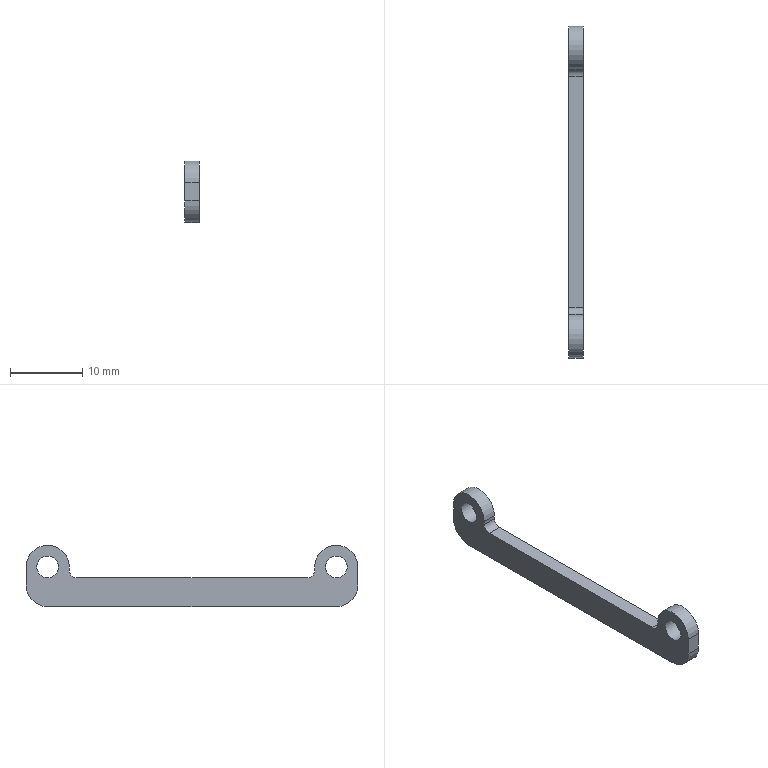Part | STEP file | 1-53.3 | 1 solid | 16 faces | box 2 x 46 x 8.5 mm | volume 425.407 mm3 | cylinder 8 | plane 8 | commonest cylinder face diameters 6 x4 2 x2 3 x2
STEP:
#1=CARTESIAN_POINT('',(0.,0.,0.));
#2=DIRECTION('',(0.,0.,1.));
#3=DIRECTION('',(1.,0.,0.));
#4=AXIS2_PLACEMENT_3D('',#1,#2,#3);
#5=CARTESIAN_POINT('',(-1.,-17.,0.));
#6=VERTEX_POINT('',#5);
#7=CARTESIAN_POINT('',(-1.,-23.,0.));
#8=VERTEX_POINT('',#7);
#9=CARTESIAN_POINT('',(-1.,-20.,0.));
#10=DIRECTION('',(1.,0.,0.));
#11=DIRECTION('',(0.,1.,0.));
#12=AXIS2_PLACEMENT_3D('',#9,#10,#11);
#13=CIRCLE('',#12,3.);
#14=CARTESIAN_POINT('',(-1.,-20.,0.));
#15=DIRECTION('',(1.,0.,0.));
#16=DIRECTION('',(0.,1.,0.));
#17=AXIS2_PLACEMENT_3D('',#14,#15,#16);
#18=CYLINDRICAL_SURFACE('',#17,3.);
#19=CARTESIAN_POINT('',(0.,0.));
#20=DIRECTION('',(1.,0.));
#21=VECTOR('',#20,1.);
#22=LINE('',#19,#21);
#23=(GEOMETRIC_REPRESENTATION_CONTEXT(2)PARAMETRIC_REPRESENTATION_CONTEXT()REPRESENTATION_CONTEXT('',''));
#24=DEFINITIONAL_REPRESENTATION('',(#22),#23);
#25=PCURVE('',#18,#24);
#26=CARTESIAN_POINT('',(-1.,0.,17.5));
#27=DIRECTION('',(1.,0.,0.));
#28=DIRECTION('',(0.,1.,0.));
#29=AXIS2_PLACEMENT_3D('',#26,#27,#28);
#30=PLANE('',#29);
#31=CARTESIAN_POINT('',(-20.,-17.5));
#32=DIRECTION('',(1.,0.));
#33=AXIS2_PLACEMENT_2D('',#31,#32);
#34=CIRCLE('',#33,3.);
#35=(GEOMETRIC_REPRESENTATION_CONTEXT(2)PARAMETRIC_REPRESENTATION_CONTEXT()REPRESENTATION_CONTEXT('',''));
#36=DEFINITIONAL_REPRESENTATION('',(#34),#35);
#37=PCURVE('',#30,#36);
#38=SURFACE_CURVE('',#13,(#25,#37),.PCURVE_S1.);
#39=EDGE_CURVE('',#6,#8,#38,.T.);
#40=ORIENTED_EDGE('',*,*,#39,.T.);
#41=CARTESIAN_POINT('',(1.,-23.,0.));
#42=VERTEX_POINT('',#41);
#43=CARTESIAN_POINT('',(-1.,-23.,0.));
#44=DIRECTION('',(1.,0.,0.));
#45=VECTOR('',#44,1.);
#46=LINE('',#43,#45);
#47=CARTESIAN_POINT('',(3.142,0.));
#48=DIRECTION('',(0.,1.));
#49=VECTOR('',#48,1.);
#50=LINE('',#47,#49);
#51=(GEOMETRIC_REPRESENTATION_CONTEXT(2)PARAMETRIC_REPRESENTATION_CONTEXT()REPRESENTATION_CONTEXT('',''));
#52=DEFINITIONAL_REPRESENTATION('',(#50),#51);
#53=PCURVE('',#18,#52);
#54=CARTESIAN_POINT('',(0.,-23.,-2.75));
#55=DIRECTION('',(0.,-1.,0.));
#56=DIRECTION('',(0.,0.,-1.));
#57=AXIS2_PLACEMENT_3D('',#54,#55,#56);
#58=PLANE('',#57);
#59=CARTESIAN_POINT('',(-2.75,-1.));
#60=DIRECTION('',(0.,1.));
#61=VECTOR('',#60,1.);
#62=LINE('',#59,#61);
#63=(GEOMETRIC_REPRESENTATION_CONTEXT(2)PARAMETRIC_REPRESENTATION_CONTEXT()REPRESENTATION_CONTEXT('',''));
#64=DEFINITIONAL_REPRESENTATION('',(#62),#63);
#65=PCURVE('',#58,#64);
#66=SURFACE_CURVE('',#46,(#53,#65),.PCURVE_S1.);
#67=EDGE_CURVE('',#8,#42,#66,.T.);
#68=ORIENTED_EDGE('',*,*,#67,.T.);
#69=CARTESIAN_POINT('',(1.,-17.,0.));
#70=VERTEX_POINT('',#69);
#71=CARTESIAN_POINT('',(1.,-20.,0.));
#72=DIRECTION('',(1.,0.,0.));
#73=DIRECTION('',(0.,1.,0.));
#74=AXIS2_PLACEMENT_3D('',#71,#72,#73);
#75=CIRCLE('',#74,3.);
#76=CARTESIAN_POINT('',(0.,2.));
#77=DIRECTION('',(1.,0.));
#78=VECTOR('',#77,1.);
#79=LINE('',#76,#78);
#80=(GEOMETRIC_REPRESENTATION_CONTEXT(2)PARAMETRIC_REPRESENTATION_CONTEXT()REPRESENTATION_CONTEXT('',''));
#81=DEFINITIONAL_REPRESENTATION('',(#79),#80);
#82=PCURVE('',#18,#81);
#83=CARTESIAN_POINT('',(1.,0.,17.5));
#84=DIRECTION('',(1.,0.,0.));
#85=DIRECTION('',(0.,1.,0.));
#86=AXIS2_PLACEMENT_3D('',#83,#84,#85);
#87=PLANE('',#86);
#88=CARTESIAN_POINT('',(-20.,-17.5));
#89=DIRECTION('',(1.,0.));
#90=AXIS2_PLACEMENT_2D('',#88,#89);
#91=CIRCLE('',#90,3.);
#92=(GEOMETRIC_REPRESENTATION_CONTEXT(2)PARAMETRIC_REPRESENTATION_CONTEXT()REPRESENTATION_CONTEXT('',''));
#93=DEFINITIONAL_REPRESENTATION('',(#91),#92);
#94=PCURVE('',#87,#93);
#95=SURFACE_CURVE('',#75,(#82,#94),.PCURVE_S1.);
#96=EDGE_CURVE('',#70,#42,#95,.T.);
#97=ORIENTED_EDGE('',*,*,#96,.F.);
#98=CARTESIAN_POINT('',(-1.,-17.,0.));
#99=DIRECTION('',(1.,0.,0.));
#100=VECTOR('',#99,1.);
#101=LINE('',#98,#100);
#102=CARTESIAN_POINT('',(0.,0.));
#103=DIRECTION('',(0.,1.));
#104=VECTOR('',#103,1.);
#105=LINE('',#102,#104);
#106=(GEOMETRIC_REPRESENTATION_CONTEXT(2)PARAMETRIC_REPRESENTATION_CONTEXT()REPRESENTATION_CONTEXT('',''));
#107=DEFINITIONAL_REPRESENTATION('',(#105),#106);
#108=PCURVE('',#18,#107);
#109=CARTESIAN_POINT('',(0.,-17.,-0.75));
#110=DIRECTION('',(0.,1.,0.));
#111=DIRECTION('',(0.,0.,1.));
#112=AXIS2_PLACEMENT_3D('',#109,#110,#111);
#113=PLANE('',#112);
#114=CARTESIAN_POINT('',(0.75,-1.));
#115=DIRECTION('',(0.,1.));
#116=VECTOR('',#115,1.);
#117=LINE('',#114,#116);
#118=(GEOMETRIC_REPRESENTATION_CONTEXT(2)PARAMETRIC_REPRESENTATION_CONTEXT()REPRESENTATION_CONTEXT('',''));
#119=DEFINITIONAL_REPRESENTATION('',(#117),#118);
#120=PCURVE('',#113,#119);
#121=SURFACE_CURVE('',#101,(#108,#120),.PCURVE_S1.);
#122=EDGE_CURVE('',#6,#70,#121,.T.);
#123=ORIENTED_EDGE('',*,*,#122,.F.);
#124=EDGE_LOOP('',(#40,#68,#97,#123));
#125=FACE_BOUND('',#124,.T.);
#126=ADVANCED_FACE('',(#125),#18,.T.);
#127=CARTESIAN_POINT('',(-1.,23.,0.));
#128=VERTEX_POINT('',#127);
#129=CARTESIAN_POINT('',(-1.,17.,0.));
#130=VERTEX_POINT('',#129);
#131=CARTESIAN_POINT('',(-1.,20.,0.));
#132=DIRECTION('',(1.,0.,0.));
#133=DIRECTION('',(0.,1.,0.));
#134=AXIS2_PLACEMENT_3D('',#131,#132,#133);
#135=CIRCLE('',#134,3.);
#136=CARTESIAN_POINT('',(-1.,20.,0.));
#137=DIRECTION('',(1.,0.,0.));
#138=DIRECTION('',(0.,1.,0.));
#139=AXIS2_PLACEMENT_3D('',#136,#137,#138);
#140=CYLINDRICAL_SURFACE('',#139,3.);
#141=CARTESIAN_POINT('',(0.,0.));
#142=DIRECTION('',(1.,0.));
#143=VECTOR('',#142,1.);
#144=LINE('',#141,#143);
#145=(GEOMETRIC_REPRESENTATION_CONTEXT(2)PARAMETRIC_REPRESENTATION_CONTEXT()REPRESENTATION_CONTEXT('',''));
#146=DEFINITIONAL_REPRESENTATION('',(#144),#145);
#147=PCURVE('',#140,#146);
#148=CARTESIAN_POINT('',(20.,-17.5));
#149=DIRECTION('',(1.,0.));
#150=AXIS2_PLACEMENT_2D('',#148,#149);
#151=CIRCLE('',#150,3.);
#152=(GEOMETRIC_REPRESENTATION_CONTEXT(2)PARAMETRIC_REPRESENTATION_CONTEXT()REPRESENTATION_CONTEXT('',''));
#153=DEFINITIONAL_REPRESENTATION('',(#151),#152);
#154=PCURVE('',#30,#153);
#155=SURFACE_CURVE('',#135,(#147,#154),.PCURVE_S1.);
#156=EDGE_CURVE('',#128,#130,#155,.T.);
#157=ORIENTED_EDGE('',*,*,#156,.T.);
#158=CARTESIAN_POINT('',(1.,17.,0.));
#159=VERTEX_POINT('',#158);
#160=CARTESIAN_POINT('',(-1.,17.,0.));
#161=DIRECTION('',(1.,0.,0.));
#162=VECTOR('',#161,1.);
#163=LINE('',#160,#162);
#164=CARTESIAN_POINT('',(3.142,0.));
#165=DIRECTION('',(0.,1.));
#166=VECTOR('',#165,1.);
#167=LINE('',#164,#166);
#168=(GEOMETRIC_REPRESENTATION_CONTEXT(2)PARAMETRIC_REPRESENTATION_CONTEXT()REPRESENTATION_CONTEXT('',''));
#169=DEFINITIONAL_REPRESENTATION('',(#167),#168);
#170=PCURVE('',#140,#169);
#171=CARTESIAN_POINT('',(0.,17.,-0.75));
#172=DIRECTION('',(0.,-1.,0.));
#173=DIRECTION('',(0.,0.,-1.));
#174=AXIS2_PLACEMENT_3D('',#171,#172,#173);
#175=PLANE('',#174);
#176=CARTESIAN_POINT('',(-0.75,-1.));
#177=DIRECTION('',(0.,1.));
#178=VECTOR('',#177,1.);
#179=LINE('',#176,#178);
#180=(GEOMETRIC_REPRESENTATION_CONTEXT(2)PARAMETRIC_REPRESENTATION_CONTEXT()REPRESENTATION_CONTEXT('',''));
#181=DEFINITIONAL_REPRESENTATION('',(#179),#180);
#182=PCURVE('',#175,#181);
#183=SURFACE_CURVE('',#163,(#170,#182),.PCURVE_S1.);
#184=EDGE_CURVE('',#130,#159,#183,.T.);
#185=ORIENTED_EDGE('',*,*,#184,.T.);
#186=CARTESIAN_POINT('',(1.,23.,0.));
#187=VERTEX_POINT('',#186);
#188=CARTESIAN_POINT('',(1.,20.,0.));
#189=DIRECTION('',(1.,0.,0.));
#190=DIRECTION('',(0.,1.,0.));
#191=AXIS2_PLACEMENT_3D('',#188,#189,#190);
#192=CIRCLE('',#191,3.);
#193=CARTESIAN_POINT('',(0.,2.));
#194=DIRECTION('',(1.,0.));
#195=VECTOR('',#194,1.);
#196=LINE('',#193,#195);
#197=(GEOMETRIC_REPRESENTATION_CONTEXT(2)PARAMETRIC_REPRESENTATION_CONTEXT()REPRESENTATION_CONTEXT('',''));
#198=DEFINITIONAL_REPRESENTATION('',(#196),#197);
#199=PCURVE('',#140,#198);
#200=CARTESIAN_POINT('',(20.,-17.5));
#201=DIRECTION('',(1.,0.));
#202=AXIS2_PLACEMENT_2D('',#200,#201);
#203=CIRCLE('',#202,3.);
#204=(GEOMETRIC_REPRESENTATION_CONTEXT(2)PARAMETRIC_REPRESENTATION_CONTEXT()REPRESENTATION_CONTEXT('',''));
#205=DEFINITIONAL_REPRESENTATION('',(#203),#204);
#206=PCURVE('',#87,#205);
#207=SURFACE_CURVE('',#192,(#199,#206),.PCURVE_S1.);
#208=EDGE_CURVE('',#187,#159,#207,.T.);
#209=ORIENTED_EDGE('',*,*,#208,.F.);
#210=CARTESIAN_POINT('',(-1.,23.,0.));
#211=DIRECTION('',(1.,0.,0.));
#212=VECTOR('',#211,1.);
#213=LINE('',#210,#212);
#214=CARTESIAN_POINT('',(0.,0.));
#215=DIRECTION('',(0.,1.));
#216=VECTOR('',#215,1.);
#217=LINE('',#214,#216);
#218=(GEOMETRIC_REPRESENTATION_CONTEXT(2)PARAMETRIC_REPRESENTATION_CONTEXT()REPRESENTATION_CONTEXT('',''));
#219=DEFINITIONAL_REPRESENTATION('',(#217),#218);
#220=PCURVE('',#140,#219);
#221=CARTESIAN_POINT('',(0.,23.,-2.75));
#222=DIRECTION('',(0.,1.,0.));
#223=DIRECTION('',(0.,0.,1.));
#224=AXIS2_PLACEMENT_3D('',#221,#222,#223);
#225=PLANE('',#224);
#226=CARTESIAN_POINT('',(2.75,-1.));
#227=DIRECTION('',(0.,1.));
#228=VECTOR('',#227,1.);
#229=LINE('',#226,#228);
#230=(GEOMETRIC_REPRESENTATION_CONTEXT(2)PARAMETRIC_REPRESENTATION_CONTEXT()REPRESENTATION_CONTEXT('',''));
#231=DEFINITIONAL_REPRESENTATION('',(#229),#230);
#232=PCURVE('',#225,#231);
#233=SURFACE_CURVE('',#213,(#220,#232),.PCURVE_S1.);
#234=EDGE_CURVE('',#128,#187,#233,.T.);
#235=ORIENTED_EDGE('',*,*,#234,.F.);
#236=EDGE_LOOP('',(#157,#185,#209,#235));
#237=FACE_BOUND('',#236,.T.);
#238=ADVANCED_FACE('',(#237),#140,.T.);
#239=CARTESIAN_POINT('',(-1.,-18.5,0.));
#240=VERTEX_POINT('',#239);
#241=CARTESIAN_POINT('',(1.,-18.5,0.));
#242=VERTEX_POINT('',#241);
#243=CARTESIAN_POINT('',(-1.,-18.5,0.));
#244=DIRECTION('',(1.,0.,0.));
#245=VECTOR('',#244,1.);
#246=LINE('',#243,#245);
#247=CARTESIAN_POINT('',(-1.,-20.,0.));
#248=DIRECTION('',(1.,0.,0.));
#249=DIRECTION('',(0.,1.,0.));
#250=AXIS2_PLACEMENT_3D('',#247,#248,#249);
#251=CYLINDRICAL_SURFACE('',#250,1.5);
#252=CARTESIAN_POINT('',(6.283,0.));
#253=DIRECTION('',(0.,1.));
#254=VECTOR('',#253,1.);
#255=LINE('',#252,#254);
#256=(GEOMETRIC_REPRESENTATION_CONTEXT(2)PARAMETRIC_REPRESENTATION_CONTEXT()REPRESENTATION_CONTEXT('',''));
#257=DEFINITIONAL_REPRESENTATION('',(#255),#256);
#258=PCURVE('',#251,#257);
#259=CARTESIAN_POINT('',(0.,0.));
#260=DIRECTION('',(0.,1.));
#261=VECTOR('',#260,1.);
#262=LINE('',#259,#261);
#263=(GEOMETRIC_REPRESENTATION_CONTEXT(2)PARAMETRIC_REPRESENTATION_CONTEXT()REPRESENTATION_CONTEXT('',''));
#264=DEFINITIONAL_REPRESENTATION('',(#262),#263);
#265=PCURVE('',#251,#264);
#266=SEAM_CURVE('',#246,(#258,#265),.PCURVE_S1.);
#267=EDGE_CURVE('',#240,#242,#266,.T.);
#268=ORIENTED_EDGE('',*,*,#267,.T.);
#269=CARTESIAN_POINT('',(1.,-20.,0.));
#270=DIRECTION('',(-1.,0.,0.));
#271=DIRECTION('',(0.,1.,0.));
#272=AXIS2_PLACEMENT_3D('',#269,#270,#271);
#273=CIRCLE('',#272,1.5);
#274=CARTESIAN_POINT('',(6.283,2.));
#275=DIRECTION('',(-1.,0.));
#276=VECTOR('',#275,1.);
#277=LINE('',#274,#276);
#278=(GEOMETRIC_REPRESENTATION_CONTEXT(2)PARAMETRIC_REPRESENTATION_CONTEXT()REPRESENTATION_CONTEXT('',''));
#279=DEFINITIONAL_REPRESENTATION('',(#277),#278);
#280=PCURVE('',#251,#279);
#281=CARTESIAN_POINT('',(-18.5,-17.5));
#282=CARTESIAN_POINT('',(-18.5,-20.098));
#283=CARTESIAN_POINT('',(-20.75,-18.799));
#284=CARTESIAN_POINT('',(-23.,-17.5));
#285=CARTESIAN_POINT('',(-20.75,-16.201));
#286=CARTESIAN_POINT('',(-18.5,-14.902));
#287=CARTESIAN_POINT('',(-18.5,-17.5));
#288=(BOUNDED_CURVE()B_SPLINE_CURVE(2,(#281,#282,#283,#284,#285,#286,#287),.UNSPECIFIED.,.T.,.F.)B_SPLINE_CURVE_WITH_KNOTS((1,2,2,2,2,1),(-2.094,0.,2.094,4.189,6.283,8.378),.UNSPECIFIED.)CURVE()GEOMETRIC_REPRESENTATION_ITEM()RATIONAL_B_SPLINE_CURVE((1.,0.5,1.,0.5,1.,0.5,1.))REPRESENTATION_ITEM(''));
#289=(GEOMETRIC_REPRESENTATION_CONTEXT(2)PARAMETRIC_REPRESENTATION_CONTEXT()REPRESENTATION_CONTEXT('',''));
#290=DEFINITIONAL_REPRESENTATION('',(#288),#289);
#291=PCURVE('',#87,#290);
#292=SURFACE_CURVE('',#273,(#280,#291),.PCURVE_S1.);
#293=EDGE_CURVE('',#242,#242,#292,.T.);
#294=ORIENTED_EDGE('',*,*,#293,.T.);
#295=ORIENTED_EDGE('',*,*,#267,.F.);
#296=CARTESIAN_POINT('',(-1.,-20.,0.));
#297=DIRECTION('',(-1.,0.,0.));
#298=DIRECTION('',(0.,1.,0.));
#299=AXIS2_PLACEMENT_3D('',#296,#297,#298);
#300=CIRCLE('',#299,1.5);
#301=CARTESIAN_POINT('',(6.283,0.));
#302=DIRECTION('',(-1.,0.));
#303=VECTOR('',#302,1.);
#304=LINE('',#301,#303);
#305=(GEOMETRIC_REPRESENTATION_CONTEXT(2)PARAMETRIC_REPRESENTATION_CONTEXT()REPRESENTATION_CONTEXT('',''));
#306=DEFINITIONAL_REPRESENTATION('',(#304),#305);
#307=PCURVE('',#251,#306);
#308=CARTESIAN_POINT('',(-18.5,-17.5));
#309=CARTESIAN_POINT('',(-18.5,-20.098));
#310=CARTESIAN_POINT('',(-20.75,-18.799));
#311=CARTESIAN_POINT('',(-23.,-17.5));
#312=CARTESIAN_POINT('',(-20.75,-16.201));
#313=CARTESIAN_POINT('',(-18.5,-14.902));
#314=CARTESIAN_POINT('',(-18.5,-17.5));
#315=(BOUNDED_CURVE()B_SPLINE_CURVE(2,(#308,#309,#310,#311,#312,#313,#314),.UNSPECIFIED.,.T.,.F.)B_SPLINE_CURVE_WITH_KNOTS((1,2,2,2,2,1),(-2.094,0.,2.094,4.189,6.283,8.378),.UNSPECIFIED.)CURVE()GEOMETRIC_REPRESENTATION_ITEM()RATIONAL_B_SPLINE_CURVE((1.,0.5,1.,0.5,1.,0.5,1.))REPRESENTATION_ITEM(''));
#316=(GEOMETRIC_REPRESENTATION_CONTEXT(2)PARAMETRIC_REPRESENTATION_CONTEXT()REPRESENTATION_CONTEXT('',''));
#317=DEFINITIONAL_REPRESENTATION('',(#315),#316);
#318=PCURVE('',#30,#317);
#319=SURFACE_CURVE('',#300,(#307,#318),.PCURVE_S1.);
#320=EDGE_CURVE('',#240,#240,#319,.T.);
#321=ORIENTED_EDGE('',*,*,#320,.F.);
#322=EDGE_LOOP('',(#268,#294,#295,#321));
#323=FACE_BOUND('',#322,.F.);
#324=ADVANCED_FACE('',(#323),#251,.F.);
#325=CARTESIAN_POINT('',(-1.,21.5,0.));
#326=VERTEX_POINT('',#325);
#327=CARTESIAN_POINT('',(1.,21.5,0.));
#328=VERTEX_POINT('',#327);
#329=CARTESIAN_POINT('',(-1.,21.5,0.));
#330=DIRECTION('',(1.,0.,0.));
#331=VECTOR('',#330,1.);
#332=LINE('',#329,#331);
#333=CARTESIAN_POINT('',(-1.,20.,0.));
#334=DIRECTION('',(1.,0.,0.));
#335=DIRECTION('',(0.,1.,0.));
#336=AXIS2_PLACEMENT_3D('',#333,#334,#335);
#337=CYLINDRICAL_SURFACE('',#336,1.5);
#338=CARTESIAN_POINT('',(6.283,0.));
#339=DIRECTION('',(0.,1.));
#340=VECTOR('',#339,1.);
#341=LINE('',#338,#340);
#342=(GEOMETRIC_REPRESENTATION_CONTEXT(2)PARAMETRIC_REPRESENTATION_CONTEXT()REPRESENTATION_CONTEXT('',''));
#343=DEFINITIONAL_REPRESENTATION('',(#341),#342);
#344=PCURVE('',#337,#343);
#345=CARTESIAN_POINT('',(0.,0.));
#346=DIRECTION('',(0.,1.));
#347=VECTOR('',#346,1.);
#348=LINE('',#345,#347);
#349=(GEOMETRIC_REPRESENTATION_CONTEXT(2)PARAMETRIC_REPRESENTATION_CONTEXT()REPRESENTATION_CONTEXT('',''));
#350=DEFINITIONAL_REPRESENTATION('',(#348),#349);
#351=PCURVE('',#337,#350);
#352=SEAM_CURVE('',#332,(#344,#351),.PCURVE_S1.);
#353=EDGE_CURVE('',#326,#328,#352,.T.);
#354=ORIENTED_EDGE('',*,*,#353,.T.);
#355=CARTESIAN_POINT('',(1.,20.,0.));
#356=DIRECTION('',(-1.,0.,0.));
#357=DIRECTION('',(0.,1.,0.));
#358=AXIS2_PLACEMENT_3D('',#355,#356,#357);
#359=CIRCLE('',#358,1.5);
#360=CARTESIAN_POINT('',(6.283,2.));
#361=DIRECTION('',(-1.,0.));
#362=VECTOR('',#361,1.);
#363=LINE('',#360,#362);
#364=(GEOMETRIC_REPRESENTATION_CONTEXT(2)PARAMETRIC_REPRESENTATION_CONTEXT()REPRESENTATION_CONTEXT('',''));
#365=DEFINITIONAL_REPRESENTATION('',(#363),#364);
#366=PCURVE('',#337,#365);
#367=CARTESIAN_POINT('',(21.5,-17.5));
#368=CARTESIAN_POINT('',(21.5,-20.098));
#369=CARTESIAN_POINT('',(19.25,-18.799));
#370=CARTESIAN_POINT('',(17.,-17.5));
#371=CARTESIAN_POINT('',(19.25,-16.201));
#372=CARTESIAN_POINT('',(21.5,-14.902));
#373=CARTESIAN_POINT('',(21.5,-17.5));
#374=(BOUNDED_CURVE()B_SPLINE_CURVE(2,(#367,#368,#369,#370,#371,#372,#373),.UNSPECIFIED.,.T.,.F.)B_SPLINE_CURVE_WITH_KNOTS((1,2,2,2,2,1),(-2.094,0.,2.094,4.189,6.283,8.378),.UNSPECIFIED.)CURVE()GEOMETRIC_REPRESENTATION_ITEM()RATIONAL_B_SPLINE_CURVE((1.,0.5,1.,0.5,1.,0.5,1.))REPRESENTATION_ITEM(''));
#375=(GEOMETRIC_REPRESENTATION_CONTEXT(2)PARAMETRIC_REPRESENTATION_CONTEXT()REPRESENTATION_CONTEXT('',''));
#376=DEFINITIONAL_REPRESENTATION('',(#374),#375);
#377=PCURVE('',#87,#376);
#378=SURFACE_CURVE('',#359,(#366,#377),.PCURVE_S1.);
#379=EDGE_CURVE('',#328,#328,#378,.T.);
#380=ORIENTED_EDGE('',*,*,#379,.T.);
#381=ORIENTED_EDGE('',*,*,#353,.F.);
#382=CARTESIAN_POINT('',(-1.,20.,0.));
#383=DIRECTION('',(-1.,0.,0.));
#384=DIRECTION('',(0.,1.,0.));
#385=AXIS2_PLACEMENT_3D('',#382,#383,#384);
#386=CIRCLE('',#385,1.5);
#387=CARTESIAN_POINT('',(6.283,0.));
#388=DIRECTION('',(-1.,0.));
#389=VECTOR('',#388,1.);
#390=LINE('',#387,#389);
#391=(GEOMETRIC_REPRESENTATION_CONTEXT(2)PARAMETRIC_REPRESENTATION_CONTEXT()REPRESENTATION_CONTEXT('',''));
#392=DEFINITIONAL_REPRESENTATION('',(#390),#391);
#393=PCURVE('',#337,#392);
#394=CARTESIAN_POINT('',(21.5,-17.5));
#395=CARTESIAN_POINT('',(21.5,-20.098));
#396=CARTESIAN_POINT('',(19.25,-18.799));
#397=CARTESIAN_POINT('',(17.,-17.5));
#398=CARTESIAN_POINT('',(19.25,-16.201));
#399=CARTESIAN_POINT('',(21.5,-14.902));
#400=CARTESIAN_POINT('',(21.5,-17.5));
#401=(BOUNDED_CURVE()B_SPLINE_CURVE(2,(#394,#395,#396,#397,#398,#399,#400),.UNSPECIFIED.,.T.,.F.)B_SPLINE_CURVE_WITH_KNOTS((1,2,2,2,2,1),(-2.094,0.,2.094,4.189,6.283,8.378),.UNSPECIFIED.)CURVE()GEOMETRIC_REPRESENTATION_ITEM()RATIONAL_B_SPLINE_CURVE((1.,0.5,1.,0.5,1.,0.5,1.))REPRESENTATION_ITEM(''));
#402=(GEOMETRIC_REPRESENTATION_CONTEXT(2)PARAMETRIC_REPRESENTATION_CONTEXT()REPRESENTATION_CONTEXT('',''));
#403=DEFINITIONAL_REPRESENTATION('',(#401),#402);
#404=PCURVE('',#30,#403);
#405=SURFACE_CURVE('',#386,(#393,#404),.PCURVE_S1.);
#406=EDGE_CURVE('',#326,#326,#405,.T.);
#407=ORIENTED_EDGE('',*,*,#406,.F.);
#408=EDGE_LOOP('',(#354,#380,#381,#407));
#409=FACE_BOUND('',#408,.F.);
#410=ADVANCED_FACE('',(#409),#337,.F.);
#411=CARTESIAN_POINT('',(-1.,-23.,-2.5));
#412=VERTEX_POINT('',#411);
#413=CARTESIAN_POINT('',(-1.,-23.,0.));
#414=DIRECTION('',(0.,0.,-1.));
#415=VECTOR('',#414,1.);
#416=LINE('',#413,#415);
#417=CARTESIAN_POINT('',(-2.75,-1.));
#418=DIRECTION('',(1.,0.));
#419=VECTOR('',#418,1.);
#420=LINE('',#417,#419);
#421=(GEOMETRIC_REPRESENTATION_CONTEXT(2)PARAMETRIC_REPRESENTATION_CONTEXT()REPRESENTATION_CONTEXT('',''));
#422=DEFINITIONAL_REPRESENTATION('',(#420),#421);
#423=PCURVE('',#58,#422);
#424=CARTESIAN_POINT('',(-23.,-17.5));
#425=DIRECTION('',(0.,-1.));
#426=VECTOR('',#425,1.);
#427=LINE('',#424,#426);
#428=(GEOMETRIC_REPRESENTATION_CONTEXT(2)PARAMETRIC_REPRESENTATION_CONTEXT()REPRESENTATION_CONTEXT('',''));
#429=DEFINITIONAL_REPRESENTATION('',(#427),#428);
#430=PCURVE('',#30,#429);
#431=SURFACE_CURVE('',#416,(#423,#430),.PCURVE_S1.);
#432=EDGE_CURVE('',#8,#412,#431,.T.);
#433=ORIENTED_EDGE('',*,*,#432,.T.);
#434=CARTESIAN_POINT('',(1.,-23.,-2.5));
#435=VERTEX_POINT('',#434);
#436=CARTESIAN_POINT('',(-1.,-23.,-2.5));
#437=DIRECTION('',(1.,0.,0.));
#438=VECTOR('',#437,1.);
#439=LINE('',#436,#438);
#440=CARTESIAN_POINT('',(-0.25,-1.));
#441=DIRECTION('',(0.,1.));
#442=VECTOR('',#441,1.);
#443=LINE('',#440,#442);
#444=(GEOMETRIC_REPRESENTATION_CONTEXT(2)PARAMETRIC_REPRESENTATION_CONTEXT()REPRESENTATION_CONTEXT('',''));
#445=DEFINITIONAL_REPRESENTATION('',(#443),#444);
#446=PCURVE('',#58,#445);
#447=CARTESIAN_POINT('',(-1.,-20.,-2.5));
#448=DIRECTION('',(1.,0.,0.));
#449=DIRECTION('',(0.,-1.,0.));
#450=AXIS2_PLACEMENT_3D('',#447,#448,#449);
#451=CYLINDRICAL_SURFACE('',#450,3.);
#452=CARTESIAN_POINT('',(0.,0.));
#453=DIRECTION('',(0.,1.));
#454=VECTOR('',#453,1.);
#455=LINE('',#452,#454);
#456=(GEOMETRIC_REPRESENTATION_CONTEXT(2)PARAMETRIC_REPRESENTATION_CONTEXT()REPRESENTATION_CONTEXT('',''));
#457=DEFINITIONAL_REPRESENTATION('',(#455),#456);
#458=PCURVE('',#451,#457);
#459=SURFACE_CURVE('',#439,(#446,#458),.PCURVE_S1.);
#460=EDGE_CURVE('',#412,#435,#459,.T.);
#461=ORIENTED_EDGE('',*,*,#460,.T.);
#462=CARTESIAN_POINT('',(1.,-23.,0.));
#463=DIRECTION('',(0.,0.,-1.));
#464=VECTOR('',#463,1.);
#465=LINE('',#462,#464);
#466=CARTESIAN_POINT('',(-2.75,1.));
#467=DIRECTION('',(1.,0.));
#468=VECTOR('',#467,1.);
#469=LINE('',#466,#468);
#470=(GEOMETRIC_REPRESENTATION_CONTEXT(2)PARAMETRIC_REPRESENTATION_CONTEXT()REPRESENTATION_CONTEXT('',''));
#471=DEFINITIONAL_REPRESENTATION('',(#469),#470);
#472=PCURVE('',#58,#471);
#473=CARTESIAN_POINT('',(-23.,-17.5));
#474=DIRECTION('',(0.,-1.));
#475=VECTOR('',#474,1.);
#476=LINE('',#473,#475);
#477=(GEOMETRIC_REPRESENTATION_CONTEXT(2)PARAMETRIC_REPRESENTATION_CONTEXT()REPRESENTATION_CONTEXT('',''));
#478=DEFINITIONAL_REPRESENTATION('',(#476),#477);
#479=PCURVE('',#87,#478);
#480=SURFACE_CURVE('',#465,(#472,#479),.PCURVE_S1.);
#481=EDGE_CURVE('',#42,#435,#480,.T.);
#482=ORIENTED_EDGE('',*,*,#481,.F.);
#483=ORIENTED_EDGE('',*,*,#67,.F.);
#484=EDGE_LOOP('',(#433,#461,#482,#483));
#485=FACE_BOUND('',#484,.T.);
#486=ADVANCED_FACE('',(#485),#58,.T.);
#487=CARTESIAN_POINT('',(-1.,-20.,-5.5));
#488=VERTEX_POINT('',#487);
#489=CARTESIAN_POINT('',(-1.,20.,-5.5));
#490=VERTEX_POINT('',#489);
#491=CARTESIAN_POINT('',(-1.,-20.,-5.5));
#492=DIRECTION('',(0.,1.,0.));
#493=VECTOR('',#492,1.);
#494=LINE('',#491,#493);
#495=CARTESIAN_POINT('',(0.,0.,-5.5));
#496=DIRECTION('',(0.,0.,-1.));
#497=DIRECTION('',(0.,1.,0.));
#498=AXIS2_PLACEMENT_3D('',#495,#496,#497);
#499=PLANE('',#498);
#500=CARTESIAN_POINT('',(-20.,-1.));
#501=DIRECTION('',(1.,0.));
#502=VECTOR('',#501,1.);
#503=LINE('',#500,#502);
#504=(GEOMETRIC_REPRESENTATION_CONTEXT(2)PARAMETRIC_REPRESENTATION_CONTEXT()REPRESENTATION_CONTEXT('',''));
#505=DEFINITIONAL_REPRESENTATION('',(#503),#504);
#506=PCURVE('',#499,#505);
#507=CARTESIAN_POINT('',(-20.,-23.));
#508=DIRECTION('',(1.,0.));
#509=VECTOR('',#508,1.);
#510=LINE('',#507,#509);
#511=(GEOMETRIC_REPRESENTATION_CONTEXT(2)PARAMETRIC_REPRESENTATION_CONTEXT()REPRESENTATION_CONTEXT('',''));
#512=DEFINITIONAL_REPRESENTATION('',(#510),#511);
#513=PCURVE('',#30,#512);
#514=SURFACE_CURVE('',#494,(#506,#513),.PCURVE_S1.);
#515=EDGE_CURVE('',#488,#490,#514,.T.);
#516=ORIENTED_EDGE('',*,*,#515,.T.);
#517=CARTESIAN_POINT('',(1.,20.,-5.5));
#518=VERTEX_POINT('',#517);
#519=CARTESIAN_POINT('',(-1.,20.,-5.5));
#520=DIRECTION('',(1.,0.,0.));
#521=VECTOR('',#520,1.);
#522=LINE('',#519,#521);
#523=CARTESIAN_POINT('',(20.,-1.));
#524=DIRECTION('',(0.,1.));
#525=VECTOR('',#524,1.);
#526=LINE('',#523,#525);
#527=(GEOMETRIC_REPRESENTATION_CONTEXT(2)PARAMETRIC_REPRESENTATION_CONTEXT()REPRESENTATION_CONTEXT('',''));
#528=DEFINITIONAL_REPRESENTATION('',(#526),#527);
#529=PCURVE('',#499,#528);
#530=CARTESIAN_POINT('',(-1.,20.,-2.5));
#531=DIRECTION('',(1.,0.,0.));
#532=DIRECTION('',(0.,0.,-1.));
#533=AXIS2_PLACEMENT_3D('',#530,#531,#532);
#534=CYLINDRICAL_SURFACE('',#533,3.);
#535=CARTESIAN_POINT('',(0.,0.));
#536=DIRECTION('',(0.,1.));
#537=VECTOR('',#536,1.);
#538=LINE('',#535,#537);
#539=(GEOMETRIC_REPRESENTATION_CONTEXT(2)PARAMETRIC_REPRESENTATION_CONTEXT()REPRESENTATION_CONTEXT('',''));
#540=DEFINITIONAL_REPRESENTATION('',(#538),#539);
#541=PCURVE('',#534,#540);
#542=SURFACE_CURVE('',#522,(#529,#541),.PCURVE_S1.);
#543=EDGE_CURVE('',#490,#518,#542,.T.);
#544=ORIENTED_EDGE('',*,*,#543,.T.);
#545=CARTESIAN_POINT('',(1.,-20.,-5.5));
#546=VERTEX_POINT('',#545);
#547=CARTESIAN_POINT('',(1.,-20.,-5.5));
#548=DIRECTION('',(0.,1.,0.));
#549=VECTOR('',#548,1.);
#550=LINE('',#547,#549);
#551=CARTESIAN_POINT('',(-20.,1.));
#552=DIRECTION('',(1.,0.));
#553=VECTOR('',#552,1.);
#554=LINE('',#551,#553);
#555=(GEOMETRIC_REPRESENTATION_CONTEXT(2)PARAMETRIC_REPRESENTATION_CONTEXT()REPRESENTATION_CONTEXT('',''));
#556=DEFINITIONAL_REPRESENTATION('',(#554),#555);
#557=PCURVE('',#499,#556);
#558=CARTESIAN_POINT('',(-20.,-23.));
#559=DIRECTION('',(1.,0.));
#560=VECTOR('',#559,1.);
#561=LINE('',#558,#560);
#562=(GEOMETRIC_REPRESENTATION_CONTEXT(2)PARAMETRIC_REPRESENTATION_CONTEXT()REPRESENTATION_CONTEXT('',''));
#563=DEFINITIONAL_REPRESENTATION('',(#561),#562);
#564=PCURVE('',#87,#563);
#565=SURFACE_CURVE('',#550,(#557,#564),.PCURVE_S1.);
#566=EDGE_CURVE('',#546,#518,#565,.T.);
#567=ORIENTED_EDGE('',*,*,#566,.F.);
#568=CARTESIAN_POINT('',(-1.,-20.,-5.5));
#569=DIRECTION('',(1.,0.,0.));
#570=VECTOR('',#569,1.);
#571=LINE('',#568,#570);
#572=CARTESIAN_POINT('',(-20.,-1.));
#573=DIRECTION('',(0.,1.));
#574=VECTOR('',#573,1.);
#575=LINE('',#572,#574);
#576=(GEOMETRIC_REPRESENTATION_CONTEXT(2)PARAMETRIC_REPRESENTATION_CONTEXT()REPRESENTATION_CONTEXT('',''));
#577=DEFINITIONAL_REPRESENTATION('',(#575),#576);
#578=PCURVE('',#499,#577);
#579=CARTESIAN_POINT('',(1.571,0.));
#580=DIRECTION('',(0.,1.));
#581=VECTOR('',#580,1.);
#582=LINE('',#579,#581);
#583=(GEOMETRIC_REPRESENTATION_CONTEXT(2)PARAMETRIC_REPRESENTATION_CONTEXT()REPRESENTATION_CONTEXT('',''));
#584=DEFINITIONAL_REPRESENTATION('',(#582),#583);
#585=PCURVE('',#451,#584);
#586=SURFACE_CURVE('',#571,(#578,#585),.PCURVE_S1.);
#587=EDGE_CURVE('',#488,#546,#586,.T.);
#588=ORIENTED_EDGE('',*,*,#587,.F.);
#589=EDGE_LOOP('',(#516,#544,#567,#588));
#590=FACE_BOUND('',#589,.T.);
#591=ADVANCED_FACE('',(#590),#499,.T.);
#592=CARTESIAN_POINT('',(1.,23.,-2.5));
#593=VERTEX_POINT('',#592);
#594=CARTESIAN_POINT('',(1.,23.,-2.5));
#595=DIRECTION('',(0.,0.,1.));
#596=VECTOR('',#595,1.);
#597=LINE('',#594,#596);
#598=CARTESIAN_POINT('',(0.25,1.));
#599=DIRECTION('',(1.,0.));
#600=VECTOR('',#599,1.);
#601=LINE('',#598,#600);
#602=(GEOMETRIC_REPRESENTATION_CONTEXT(2)PARAMETRIC_REPRESENTATION_CONTEXT()REPRESENTATION_CONTEXT('',''));
#603=DEFINITIONAL_REPRESENTATION('',(#601),#602);
#604=PCURVE('',#225,#603);
#605=CARTESIAN_POINT('',(23.,-20.));
#606=DIRECTION('',(0.,1.));
#607=VECTOR('',#606,1.);
#608=LINE('',#605,#607);
#609=(GEOMETRIC_REPRESENTATION_CONTEXT(2)PARAMETRIC_REPRESENTATION_CONTEXT()REPRESENTATION_CONTEXT('',''));
#610=DEFINITIONAL_REPRESENTATION('',(#608),#609);
#611=PCURVE('',#87,#610);
#612=SURFACE_CURVE('',#597,(#604,#611),.PCURVE_S1.);
#613=EDGE_CURVE('',#593,#187,#612,.T.);
#614=ORIENTED_EDGE('',*,*,#613,.F.);
#615=CARTESIAN_POINT('',(-1.,23.,-2.5));
#616=VERTEX_POINT('',#615);
#617=CARTESIAN_POINT('',(-1.,23.,-2.5));
#618=DIRECTION('',(1.,0.,0.));
#619=VECTOR('',#618,1.);
#620=LINE('',#617,#619);
#621=CARTESIAN_POINT('',(0.25,-1.));
#622=DIRECTION('',(0.,1.));
#623=VECTOR('',#622,1.);
#624=LINE('',#621,#623);
#625=(GEOMETRIC_REPRESENTATION_CONTEXT(2)PARAMETRIC_REPRESENTATION_CONTEXT()REPRESENTATION_CONTEXT('',''));
#626=DEFINITIONAL_REPRESENTATION('',(#624),#625);
#627=PCURVE('',#225,#626);
#628=CARTESIAN_POINT('',(1.571,0.));
#629=DIRECTION('',(0.,1.));
#630=VECTOR('',#629,1.);
#631=LINE('',#628,#630);
#632=(GEOMETRIC_REPRESENTATION_CONTEXT(2)PARAMETRIC_REPRESENTATION_CONTEXT()REPRESENTATION_CONTEXT('',''));
#633=DEFINITIONAL_REPRESENTATION('',(#631),#632);
#634=PCURVE('',#534,#633);
#635=SURFACE_CURVE('',#620,(#627,#634),.PCURVE_S1.);
#636=EDGE_CURVE('',#616,#593,#635,.T.);
#637=ORIENTED_EDGE('',*,*,#636,.F.);
#638=CARTESIAN_POINT('',(-1.,23.,-2.5));
#639=DIRECTION('',(0.,0.,1.));
#640=VECTOR('',#639,1.);
#641=LINE('',#638,#640);
#642=CARTESIAN_POINT('',(0.25,-1.));
#643=DIRECTION('',(1.,0.));
#644=VECTOR('',#643,1.);
#645=LINE('',#642,#644);
#646=(GEOMETRIC_REPRESENTATION_CONTEXT(2)PARAMETRIC_REPRESENTATION_CONTEXT()REPRESENTATION_CONTEXT('',''));
#647=DEFINITIONAL_REPRESENTATION('',(#645),#646);
#648=PCURVE('',#225,#647);
#649=CARTESIAN_POINT('',(23.,-20.));
#650=DIRECTION('',(0.,1.));
#651=VECTOR('',#650,1.);
#652=LINE('',#649,#651);
#653=(GEOMETRIC_REPRESENTATION_CONTEXT(2)PARAMETRIC_REPRESENTATION_CONTEXT()REPRESENTATION_CONTEXT('',''));
#654=DEFINITIONAL_REPRESENTATION('',(#652),#653);
#655=PCURVE('',#30,#654);
#656=SURFACE_CURVE('',#641,(#648,#655),.PCURVE_S1.);
#657=EDGE_CURVE('',#616,#128,#656,.T.);
#658=ORIENTED_EDGE('',*,*,#657,.T.);
#659=ORIENTED_EDGE('',*,*,#234,.T.);
#660=EDGE_LOOP('',(#614,#637,#658,#659));
#661=FACE_BOUND('',#660,.T.);
#662=ADVANCED_FACE('',(#661),#225,.T.);
#663=CARTESIAN_POINT('',(-1.,-20.,-2.5));
#664=DIRECTION('',(1.,0.,0.));
#665=DIRECTION('',(0.,-1.,0.));
#666=AXIS2_PLACEMENT_3D('',#663,#664,#665);
#667=CIRCLE('',#666,3.);
#668=CARTESIAN_POINT('',(0.,0.));
#669=DIRECTION('',(1.,0.));
#670=VECTOR('',#669,1.);
#671=LINE('',#668,#670);
#672=(GEOMETRIC_REPRESENTATION_CONTEXT(2)PARAMETRIC_REPRESENTATION_CONTEXT()REPRESENTATION_CONTEXT('',''));
#673=DEFINITIONAL_REPRESENTATION('',(#671),#672);
#674=PCURVE('',#451,#673);
#675=CARTESIAN_POINT('',(-20.,-20.));
#676=DIRECTION('',(-1.,0.));
#677=AXIS2_PLACEMENT_2D('',#675,#676);
#678=CIRCLE('',#677,3.);
#679=(GEOMETRIC_REPRESENTATION_CONTEXT(2)PARAMETRIC_REPRESENTATION_CONTEXT()REPRESENTATION_CONTEXT('',''));
#680=DEFINITIONAL_REPRESENTATION('',(#678),#679);
#681=PCURVE('',#30,#680);
#682=SURFACE_CURVE('',#667,(#674,#681),.PCURVE_S1.);
#683=EDGE_CURVE('',#412,#488,#682,.T.);
#684=ORIENTED_EDGE('',*,*,#683,.T.);
#685=ORIENTED_EDGE('',*,*,#587,.T.);
#686=CARTESIAN_POINT('',(1.,-20.,-2.5));
#687=DIRECTION('',(1.,0.,0.));
#688=DIRECTION('',(0.,-1.,0.));
#689=AXIS2_PLACEMENT_3D('',#686,#687,#688);
#690=CIRCLE('',#689,3.);
#691=CARTESIAN_POINT('',(0.,2.));
#692=DIRECTION('',(1.,0.));
#693=VECTOR('',#692,1.);
#694=LINE('',#691,#693);
#695=(GEOMETRIC_REPRESENTATION_CONTEXT(2)PARAMETRIC_REPRESENTATION_CONTEXT()REPRESENTATION_CONTEXT('',''));
#696=DEFINITIONAL_REPRESENTATION('',(#694),#695);
#697=PCURVE('',#451,#696);
#698=CARTESIAN_POINT('',(-20.,-20.));
#699=DIRECTION('',(-1.,0.));
#700=AXIS2_PLACEMENT_2D('',#698,#699);
#701=CIRCLE('',#700,3.);
#702=(GEOMETRIC_REPRESENTATION_CONTEXT(2)PARAMETRIC_REPRESENTATION_CONTEXT()REPRESENTATION_CONTEXT('',''));
#703=DEFINITIONAL_REPRESENTATION('',(#701),#702);
#704=PCURVE('',#87,#703);
#705=SURFACE_CURVE('',#690,(#697,#704),.PCURVE_S1.);
#706=EDGE_CURVE('',#435,#546,#705,.T.);
#707=ORIENTED_EDGE('',*,*,#706,.F.);
#708=ORIENTED_EDGE('',*,*,#460,.F.);
#709=EDGE_LOOP('',(#684,#685,#707,#708));
#710=FACE_BOUND('',#709,.T.);
#711=ADVANCED_FACE('',(#710),#451,.T.);
#712=CARTESIAN_POINT('',(-1.,20.,-2.5));
#713=DIRECTION('',(1.,0.,0.));
#714=DIRECTION('',(0.,0.,-1.));
#715=AXIS2_PLACEMENT_3D('',#712,#713,#714);
#716=CIRCLE('',#715,3.);
#717=CARTESIAN_POINT('',(0.,0.));
#718=DIRECTION('',(1.,0.));
#719=VECTOR('',#718,1.);
#720=LINE('',#717,#719);
#721=(GEOMETRIC_REPRESENTATION_CONTEXT(2)PARAMETRIC_REPRESENTATION_CONTEXT()REPRESENTATION_CONTEXT('',''));
#722=DEFINITIONAL_REPRESENTATION('',(#720),#721);
#723=PCURVE('',#534,#722);
#724=CARTESIAN_POINT('',(20.,-20.));
#725=DIRECTION('',(0.,-1.));
#726=AXIS2_PLACEMENT_2D('',#724,#725);
#727=CIRCLE('',#726,3.);
#728=(GEOMETRIC_REPRESENTATION_CONTEXT(2)PARAMETRIC_REPRESENTATION_CONTEXT()REPRESENTATION_CONTEXT('',''));
#729=DEFINITIONAL_REPRESENTATION('',(#727),#728);
#730=PCURVE('',#30,#729);
#731=SURFACE_CURVE('',#716,(#723,#730),.PCURVE_S1.);
#732=EDGE_CURVE('',#490,#616,#731,.T.);
#733=ORIENTED_EDGE('',*,*,#732,.T.);
#734=ORIENTED_EDGE('',*,*,#636,.T.);
#735=CARTESIAN_POINT('',(1.,20.,-2.5));
#736=DIRECTION('',(1.,0.,0.));
#737=DIRECTION('',(0.,0.,-1.));
#738=AXIS2_PLACEMENT_3D('',#735,#736,#737);
#739=CIRCLE('',#738,3.);
#740=CARTESIAN_POINT('',(0.,2.));
#741=DIRECTION('',(1.,0.));
#742=VECTOR('',#741,1.);
#743=LINE('',#740,#742);
#744=(GEOMETRIC_REPRESENTATION_CONTEXT(2)PARAMETRIC_REPRESENTATION_CONTEXT()REPRESENTATION_CONTEXT('',''));
#745=DEFINITIONAL_REPRESENTATION('',(#743),#744);
#746=PCURVE('',#534,#745);
#747=CARTESIAN_POINT('',(20.,-20.));
#748=DIRECTION('',(0.,-1.));
#749=AXIS2_PLACEMENT_2D('',#747,#748);
#750=CIRCLE('',#749,3.);
#751=(GEOMETRIC_REPRESENTATION_CONTEXT(2)PARAMETRIC_REPRESENTATION_CONTEXT()REPRESENTATION_CONTEXT('',''));
#752=DEFINITIONAL_REPRESENTATION('',(#750),#751);
#753=PCURVE('',#87,#752);
#754=SURFACE_CURVE('',#739,(#746,#753),.PCURVE_S1.);
#755=EDGE_CURVE('',#518,#593,#754,.T.);
#756=ORIENTED_EDGE('',*,*,#755,.F.);
#757=ORIENTED_EDGE('',*,*,#543,.F.);
#758=EDGE_LOOP('',(#733,#734,#756,#757));
#759=FACE_BOUND('',#758,.T.);
#760=ADVANCED_FACE('',(#759),#534,.T.);
#761=CARTESIAN_POINT('',(-1.,17.,-0.5));
#762=VERTEX_POINT('',#761);
#763=CARTESIAN_POINT('',(-1.,17.,0.));
#764=DIRECTION('',(0.,0.,-1.));
#765=VECTOR('',#764,1.);
#766=LINE('',#763,#765);
#767=CARTESIAN_POINT('',(-0.75,-1.));
#768=DIRECTION('',(1.,0.));
#769=VECTOR('',#768,1.);
#770=LINE('',#767,#769);
#771=(GEOMETRIC_REPRESENTATION_CONTEXT(2)PARAMETRIC_REPRESENTATION_CONTEXT()REPRESENTATION_CONTEXT('',''));
#772=DEFINITIONAL_REPRESENTATION('',(#770),#771);
#773=PCURVE('',#175,#772);
#774=CARTESIAN_POINT('',(17.,-17.5));
#775=DIRECTION('',(0.,-1.));
#776=VECTOR('',#775,1.);
#777=LINE('',#774,#776);
#778=(GEOMETRIC_REPRESENTATION_CONTEXT(2)PARAMETRIC_REPRESENTATION_CONTEXT()REPRESENTATION_CONTEXT('',''));
#779=DEFINITIONAL_REPRESENTATION('',(#777),#778);
#780=PCURVE('',#30,#779);
#781=SURFACE_CURVE('',#766,(#773,#780),.PCURVE_S1.);
#782=EDGE_CURVE('',#130,#762,#781,.T.);
#783=ORIENTED_EDGE('',*,*,#782,.T.);
#784=CARTESIAN_POINT('',(1.,17.,-0.5));
#785=VERTEX_POINT('',#784);
#786=CARTESIAN_POINT('',(-1.,17.,-0.5));
#787=DIRECTION('',(1.,0.,0.));
#788=VECTOR('',#787,1.);
#789=LINE('',#786,#788);
#790=CARTESIAN_POINT('',(-0.25,-1.));
#791=DIRECTION('',(0.,1.));
#792=VECTOR('',#791,1.);
#793=LINE('',#790,#792);
#794=(GEOMETRIC_REPRESENTATION_CONTEXT(2)PARAMETRIC_REPRESENTATION_CONTEXT()REPRESENTATION_CONTEXT('',''));
#795=DEFINITIONAL_REPRESENTATION('',(#793),#794);
#796=PCURVE('',#175,#795);
#797=CARTESIAN_POINT('',(-1.,16.,-0.5));
#798=DIRECTION('',(1.,0.,0.));
#799=DIRECTION('',(0.,1.,0.));
#800=AXIS2_PLACEMENT_3D('',#797,#798,#799);
#801=CYLINDRICAL_SURFACE('',#800,1.);
#802=CARTESIAN_POINT('',(6.283,0.));
#803=DIRECTION('',(0.,1.));
#804=VECTOR('',#803,1.);
#805=LINE('',#802,#804);
#806=(GEOMETRIC_REPRESENTATION_CONTEXT(2)PARAMETRIC_REPRESENTATION_CONTEXT()REPRESENTATION_CONTEXT('',''));
#807=DEFINITIONAL_REPRESENTATION('',(#805),#806);
#808=PCURVE('',#801,#807);
#809=SURFACE_CURVE('',#789,(#796,#808),.PCURVE_S1.);
#810=EDGE_CURVE('',#762,#785,#809,.T.);
#811=ORIENTED_EDGE('',*,*,#810,.T.);
#812=CARTESIAN_POINT('',(1.,17.,0.));
#813=DIRECTION('',(0.,0.,-1.));
#814=VECTOR('',#813,1.);
#815=LINE('',#812,#814);
#816=CARTESIAN_POINT('',(-0.75,1.));
#817=DIRECTION('',(1.,0.));
#818=VECTOR('',#817,1.);
#819=LINE('',#816,#818);
#820=(GEOMETRIC_REPRESENTATION_CONTEXT(2)PARAMETRIC_REPRESENTATION_CONTEXT()REPRESENTATION_CONTEXT('',''));
#821=DEFINITIONAL_REPRESENTATION('',(#819),#820);
#822=PCURVE('',#175,#821);
#823=CARTESIAN_POINT('',(17.,-17.5));
#824=DIRECTION('',(0.,-1.));
#825=VECTOR('',#824,1.);
#826=LINE('',#823,#825);
#827=(GEOMETRIC_REPRESENTATION_CONTEXT(2)PARAMETRIC_REPRESENTATION_CONTEXT()REPRESENTATION_CONTEXT('',''));
#828=DEFINITIONAL_REPRESENTATION('',(#826),#827);
#829=PCURVE('',#87,#828);
#830=SURFACE_CURVE('',#815,(#822,#829),.PCURVE_S1.);
#831=EDGE_CURVE('',#159,#785,#830,.T.);
#832=ORIENTED_EDGE('',*,*,#831,.F.);
#833=ORIENTED_EDGE('',*,*,#184,.F.);
#834=EDGE_LOOP('',(#783,#811,#832,#833));
#835=FACE_BOUND('',#834,.T.);
#836=ADVANCED_FACE('',(#835),#175,.T.);
#837=CARTESIAN_POINT('',(-1.,16.,-1.5));
#838=VERTEX_POINT('',#837);
#839=CARTESIAN_POINT('',(-1.,-16.,-1.5));
#840=VERTEX_POINT('',#839);
#841=CARTESIAN_POINT('',(-1.,16.,-1.5));
#842=DIRECTION('',(0.,-1.,0.));
#843=VECTOR('',#842,1.);
#844=LINE('',#841,#843);
#845=CARTESIAN_POINT('',(0.,0.,-1.5));
#846=DIRECTION('',(0.,0.,1.));
#847=DIRECTION('',(0.,-1.,0.));
#848=AXIS2_PLACEMENT_3D('',#845,#846,#847);
#849=PLANE('',#848);
#850=CARTESIAN_POINT('',(-16.,-1.));
#851=DIRECTION('',(1.,0.));
#852=VECTOR('',#851,1.);
#853=LINE('',#850,#852);
#854=(GEOMETRIC_REPRESENTATION_CONTEXT(2)PARAMETRIC_REPRESENTATION_CONTEXT()REPRESENTATION_CONTEXT('',''));
#855=DEFINITIONAL_REPRESENTATION('',(#853),#854);
#856=PCURVE('',#849,#855);
#857=CARTESIAN_POINT('',(16.,-19.));
#858=DIRECTION('',(-1.,0.));
#859=VECTOR('',#858,1.);
#860=LINE('',#857,#859);
#861=(GEOMETRIC_REPRESENTATION_CONTEXT(2)PARAMETRIC_REPRESENTATION_CONTEXT()REPRESENTATION_CONTEXT('',''));
#862=DEFINITIONAL_REPRESENTATION('',(#860),#861);
#863=PCURVE('',#30,#862);
#864=SURFACE_CURVE('',#844,(#856,#863),.PCURVE_S1.);
#865=EDGE_CURVE('',#838,#840,#864,.T.);
#866=ORIENTED_EDGE('',*,*,#865,.T.);
#867=CARTESIAN_POINT('',(1.,-16.,-1.5));
#868=VERTEX_POINT('',#867);
#869=CARTESIAN_POINT('',(-1.,-16.,-1.5));
#870=DIRECTION('',(1.,0.,0.));
#871=VECTOR('',#870,1.);
#872=LINE('',#869,#871);
#873=CARTESIAN_POINT('',(16.,-1.));
#874=DIRECTION('',(0.,1.));
#875=VECTOR('',#874,1.);
#876=LINE('',#873,#875);
#877=(GEOMETRIC_REPRESENTATION_CONTEXT(2)PARAMETRIC_REPRESENTATION_CONTEXT()REPRESENTATION_CONTEXT('',''));
#878=DEFINITIONAL_REPRESENTATION('',(#876),#877);
#879=PCURVE('',#849,#878);
#880=CARTESIAN_POINT('',(-1.,-16.,-0.5));
#881=DIRECTION('',(1.,0.,0.));
#882=DIRECTION('',(0.,0.,-1.));
#883=AXIS2_PLACEMENT_3D('',#880,#881,#882);
#884=CYLINDRICAL_SURFACE('',#883,1.);
#885=CARTESIAN_POINT('',(6.283,0.));
#886=DIRECTION('',(0.,1.));
#887=VECTOR('',#886,1.);
#888=LINE('',#885,#887);
#889=(GEOMETRIC_REPRESENTATION_CONTEXT(2)PARAMETRIC_REPRESENTATION_CONTEXT()REPRESENTATION_CONTEXT('',''));
#890=DEFINITIONAL_REPRESENTATION('',(#888),#889);
#891=PCURVE('',#884,#890);
#892=SURFACE_CURVE('',#872,(#879,#891),.PCURVE_S1.);
#893=EDGE_CURVE('',#840,#868,#892,.T.);
#894=ORIENTED_EDGE('',*,*,#893,.T.);
#895=CARTESIAN_POINT('',(1.,16.,-1.5));
#896=VERTEX_POINT('',#895);
#897=CARTESIAN_POINT('',(1.,16.,-1.5));
#898=DIRECTION('',(0.,-1.,0.));
#899=VECTOR('',#898,1.);
#900=LINE('',#897,#899);
#901=CARTESIAN_POINT('',(-16.,1.));
#902=DIRECTION('',(1.,0.));
#903=VECTOR('',#902,1.);
#904=LINE('',#901,#903);
#905=(GEOMETRIC_REPRESENTATION_CONTEXT(2)PARAMETRIC_REPRESENTATION_CONTEXT()REPRESENTATION_CONTEXT('',''));
#906=DEFINITIONAL_REPRESENTATION('',(#904),#905);
#907=PCURVE('',#849,#906);
#908=CARTESIAN_POINT('',(16.,-19.));
#909=DIRECTION('',(-1.,0.));
#910=VECTOR('',#909,1.);
#911=LINE('',#908,#910);
#912=(GEOMETRIC_REPRESENTATION_CONTEXT(2)PARAMETRIC_REPRESENTATION_CONTEXT()REPRESENTATION_CONTEXT('',''));
#913=DEFINITIONAL_REPRESENTATION('',(#911),#912);
#914=PCURVE('',#87,#913);
#915=SURFACE_CURVE('',#900,(#907,#914),.PCURVE_S1.);
#916=EDGE_CURVE('',#896,#868,#915,.T.);
#917=ORIENTED_EDGE('',*,*,#916,.F.);
#918=CARTESIAN_POINT('',(-1.,16.,-1.5));
#919=DIRECTION('',(1.,0.,0.));
#920=VECTOR('',#919,1.);
#921=LINE('',#918,#920);
#922=CARTESIAN_POINT('',(-16.,-1.));
#923=DIRECTION('',(0.,1.));
#924=VECTOR('',#923,1.);
#925=LINE('',#922,#924);
#926=(GEOMETRIC_REPRESENTATION_CONTEXT(2)PARAMETRIC_REPRESENTATION_CONTEXT()REPRESENTATION_CONTEXT('',''));
#927=DEFINITIONAL_REPRESENTATION('',(#925),#926);
#928=PCURVE('',#849,#927);
#929=CARTESIAN_POINT('',(4.712,0.));
#930=DIRECTION('',(0.,1.));
#931=VECTOR('',#930,1.);
#932=LINE('',#929,#931);
#933=(GEOMETRIC_REPRESENTATION_CONTEXT(2)PARAMETRIC_REPRESENTATION_CONTEXT()REPRESENTATION_CONTEXT('',''));
#934=DEFINITIONAL_REPRESENTATION('',(#932),#933);
#935=PCURVE('',#801,#934);
#936=SURFACE_CURVE('',#921,(#928,#935),.PCURVE_S1.);
#937=EDGE_CURVE('',#838,#896,#936,.T.);
#938=ORIENTED_EDGE('',*,*,#937,.F.);
#939=EDGE_LOOP('',(#866,#894,#917,#938));
#940=FACE_BOUND('',#939,.T.);
#941=ADVANCED_FACE('',(#940),#849,.T.);
#942=CARTESIAN_POINT('',(1.,-17.,-0.5));
#943=VERTEX_POINT('',#942);
#944=CARTESIAN_POINT('',(1.,-17.,-0.5));
#945=DIRECTION('',(0.,0.,1.));
#946=VECTOR('',#945,1.);
#947=LINE('',#944,#946);
#948=CARTESIAN_POINT('',(0.25,1.));
#949=DIRECTION('',(1.,0.));
#950=VECTOR('',#949,1.);
#951=LINE('',#948,#950);
#952=(GEOMETRIC_REPRESENTATION_CONTEXT(2)PARAMETRIC_REPRESENTATION_CONTEXT()REPRESENTATION_CONTEXT('',''));
#953=DEFINITIONAL_REPRESENTATION('',(#951),#952);
#954=PCURVE('',#113,#953);
#955=CARTESIAN_POINT('',(-17.,-18.));
#956=DIRECTION('',(0.,1.));
#957=VECTOR('',#956,1.);
#958=LINE('',#955,#957);
#959=(GEOMETRIC_REPRESENTATION_CONTEXT(2)PARAMETRIC_REPRESENTATION_CONTEXT()REPRESENTATION_CONTEXT('',''));
#960=DEFINITIONAL_REPRESENTATION('',(#958),#959);
#961=PCURVE('',#87,#960);
#962=SURFACE_CURVE('',#947,(#954,#961),.PCURVE_S1.);
#963=EDGE_CURVE('',#943,#70,#962,.T.);
#964=ORIENTED_EDGE('',*,*,#963,.F.);
#965=CARTESIAN_POINT('',(-1.,-17.,-0.5));
#966=VERTEX_POINT('',#965);
#967=CARTESIAN_POINT('',(-1.,-17.,-0.5));
#968=DIRECTION('',(1.,0.,0.));
#969=VECTOR('',#968,1.);
#970=LINE('',#967,#969);
#971=CARTESIAN_POINT('',(0.25,-1.));
#972=DIRECTION('',(0.,1.));
#973=VECTOR('',#972,1.);
#974=LINE('',#971,#973);
#975=(GEOMETRIC_REPRESENTATION_CONTEXT(2)PARAMETRIC_REPRESENTATION_CONTEXT()REPRESENTATION_CONTEXT('',''));
#976=DEFINITIONAL_REPRESENTATION('',(#974),#975);
#977=PCURVE('',#113,#976);
#978=CARTESIAN_POINT('',(4.712,0.));
#979=DIRECTION('',(0.,1.));
#980=VECTOR('',#979,1.);
#981=LINE('',#978,#980);
#982=(GEOMETRIC_REPRESENTATION_CONTEXT(2)PARAMETRIC_REPRESENTATION_CONTEXT()REPRESENTATION_CONTEXT('',''));
#983=DEFINITIONAL_REPRESENTATION('',(#981),#982);
#984=PCURVE('',#884,#983);
#985=SURFACE_CURVE('',#970,(#977,#984),.PCURVE_S1.);
#986=EDGE_CURVE('',#966,#943,#985,.T.);
#987=ORIENTED_EDGE('',*,*,#986,.F.);
#988=CARTESIAN_POINT('',(-1.,-17.,-0.5));
#989=DIRECTION('',(0.,0.,1.));
#990=VECTOR('',#989,1.);
#991=LINE('',#988,#990);
#992=CARTESIAN_POINT('',(0.25,-1.));
#993=DIRECTION('',(1.,0.));
#994=VECTOR('',#993,1.);
#995=LINE('',#992,#994);
#996=(GEOMETRIC_REPRESENTATION_CONTEXT(2)PARAMETRIC_REPRESENTATION_CONTEXT()REPRESENTATION_CONTEXT('',''));
#997=DEFINITIONAL_REPRESENTATION('',(#995),#996);
#998=PCURVE('',#113,#997);
#999=CARTESIAN_POINT('',(-17.,-18.));
#1000=DIRECTION('',(0.,1.));
#1001=VECTOR('',#1000,1.);
#1002=LINE('',#999,#1001);
#1003=(GEOMETRIC_REPRESENTATION_CONTEXT(2)PARAMETRIC_REPRESENTATION_CONTEXT()REPRESENTATION_CONTEXT('',''));
#1004=DEFINITIONAL_REPRESENTATION('',(#1002),#1003);
#1005=PCURVE('',#30,#1004);
#1006=SURFACE_CURVE('',#991,(#998,#1005),.PCURVE_S1.);
#1007=EDGE_CURVE('',#966,#6,#1006,.T.);
#1008=ORIENTED_EDGE('',*,*,#1007,.T.);
#1009=ORIENTED_EDGE('',*,*,#122,.T.);
#1010=EDGE_LOOP('',(#964,#987,#1008,#1009));
#1011=FACE_BOUND('',#1010,.T.);
#1012=ADVANCED_FACE('',(#1011),#113,.T.);
#1013=ORIENTED_EDGE('',*,*,#1007,.T.);
#1014=ORIENTED_EDGE('',*,*,#39,.T.);
#1015=ORIENTED_EDGE('',*,*,#432,.T.);
#1016=ORIENTED_EDGE('',*,*,#683,.T.);
#1017=ORIENTED_EDGE('',*,*,#515,.T.);
#1018=ORIENTED_EDGE('',*,*,#732,.T.);
#1019=ORIENTED_EDGE('',*,*,#657,.T.);
#1020=ORIENTED_EDGE('',*,*,#156,.T.);
#1021=ORIENTED_EDGE('',*,*,#782,.T.);
#1022=CARTESIAN_POINT('',(-1.,16.,-0.5));
#1023=DIRECTION('',(-1.,0.,0.));
#1024=DIRECTION('',(0.,1.,0.));
#1025=AXIS2_PLACEMENT_3D('',#1022,#1023,#1024);
#1026=CIRCLE('',#1025,1.);
#1027=CARTESIAN_POINT('',(17.,-18.));
#1028=CARTESIAN_POINT('',(17.,-19.732));
#1029=CARTESIAN_POINT('',(15.5,-18.866));
#1030=CARTESIAN_POINT('',(14.,-18.));
#1031=CARTESIAN_POINT('',(15.5,-17.134));
#1032=CARTESIAN_POINT('',(17.,-16.268));
#1033=CARTESIAN_POINT('',(17.,-18.));
#1034=(BOUNDED_CURVE()B_SPLINE_CURVE(2,(#1027,#1028,#1029,#1030,#1031,#1032,#1033),.UNSPECIFIED.,.T.,.F.)B_SPLINE_CURVE_WITH_KNOTS((1,2,2,2,2,1),(-2.094,0.,2.094,4.189,6.283,8.378),.UNSPECIFIED.)CURVE()GEOMETRIC_REPRESENTATION_ITEM()RATIONAL_B_SPLINE_CURVE((1.,0.5,1.,0.5,1.,0.5,1.))REPRESENTATION_ITEM(''));
#1035=(GEOMETRIC_REPRESENTATION_CONTEXT(2)PARAMETRIC_REPRESENTATION_CONTEXT()REPRESENTATION_CONTEXT('',''));
#1036=DEFINITIONAL_REPRESENTATION('',(#1034),#1035);
#1037=PCURVE('',#30,#1036);
#1038=CARTESIAN_POINT('',(6.283,0.));
#1039=DIRECTION('',(-1.,0.));
#1040=VECTOR('',#1039,1.);
#1041=LINE('',#1038,#1040);
#1042=(GEOMETRIC_REPRESENTATION_CONTEXT(2)PARAMETRIC_REPRESENTATION_CONTEXT()REPRESENTATION_CONTEXT('',''));
#1043=DEFINITIONAL_REPRESENTATION('',(#1041),#1042);
#1044=PCURVE('',#801,#1043);
#1045=SURFACE_CURVE('',#1026,(#1037,#1044),.PCURVE_S1.);
#1046=EDGE_CURVE('',#762,#838,#1045,.T.);
#1047=ORIENTED_EDGE('',*,*,#1046,.T.);
#1048=ORIENTED_EDGE('',*,*,#865,.T.);
#1049=CARTESIAN_POINT('',(-1.,-16.,-0.5));
#1050=DIRECTION('',(-1.,0.,0.));
#1051=DIRECTION('',(0.,0.,-1.));
#1052=AXIS2_PLACEMENT_3D('',#1049,#1050,#1051);
#1053=CIRCLE('',#1052,1.);
#1054=CARTESIAN_POINT('',(-16.,-19.));
#1055=CARTESIAN_POINT('',(-17.732,-19.));
#1056=CARTESIAN_POINT('',(-16.866,-17.5));
#1057=CARTESIAN_POINT('',(-16.,-16.));
#1058=CARTESIAN_POINT('',(-15.134,-17.5));
#1059=CARTESIAN_POINT('',(-14.268,-19.));
#1060=CARTESIAN_POINT('',(-16.,-19.));
#1061=(BOUNDED_CURVE()B_SPLINE_CURVE(2,(#1054,#1055,#1056,#1057,#1058,#1059,#1060),.UNSPECIFIED.,.T.,.F.)B_SPLINE_CURVE_WITH_KNOTS((1,2,2,2,2,1),(-2.094,0.,2.094,4.189,6.283,8.378),.UNSPECIFIED.)CURVE()GEOMETRIC_REPRESENTATION_ITEM()RATIONAL_B_SPLINE_CURVE((1.,0.5,1.,0.5,1.,0.5,1.))REPRESENTATION_ITEM(''));
#1062=(GEOMETRIC_REPRESENTATION_CONTEXT(2)PARAMETRIC_REPRESENTATION_CONTEXT()REPRESENTATION_CONTEXT('',''));
#1063=DEFINITIONAL_REPRESENTATION('',(#1061),#1062);
#1064=PCURVE('',#30,#1063);
#1065=CARTESIAN_POINT('',(6.283,0.));
#1066=DIRECTION('',(-1.,0.));
#1067=VECTOR('',#1066,1.);
#1068=LINE('',#1065,#1067);
#1069=(GEOMETRIC_REPRESENTATION_CONTEXT(2)PARAMETRIC_REPRESENTATION_CONTEXT()REPRESENTATION_CONTEXT('',''));
#1070=DEFINITIONAL_REPRESENTATION('',(#1068),#1069);
#1071=PCURVE('',#884,#1070);
#1072=SURFACE_CURVE('',#1053,(#1064,#1071),.PCURVE_S1.);
#1073=EDGE_CURVE('',#840,#966,#1072,.T.);
#1074=ORIENTED_EDGE('',*,*,#1073,.T.);
#1075=EDGE_LOOP('',(#1013,#1014,#1015,#1016,#1017,#1018,#1019,#1020,#1021,#1047,#1048,#1074));
#1076=FACE_BOUND('',#1075,.F.);
#1077=ORIENTED_EDGE('',*,*,#320,.T.);
#1078=EDGE_LOOP('',(#1077));
#1079=FACE_BOUND('',#1078,.F.);
#1080=ORIENTED_EDGE('',*,*,#406,.T.);
#1081=EDGE_LOOP('',(#1080));
#1082=FACE_BOUND('',#1081,.F.);
#1083=ADVANCED_FACE('',(#1076,#1079,#1082),#30,.F.);
#1084=ORIENTED_EDGE('',*,*,#963,.T.);
#1085=ORIENTED_EDGE('',*,*,#96,.T.);
#1086=ORIENTED_EDGE('',*,*,#481,.T.);
#1087=ORIENTED_EDGE('',*,*,#706,.T.);
#1088=ORIENTED_EDGE('',*,*,#566,.T.);
#1089=ORIENTED_EDGE('',*,*,#755,.T.);
#1090=ORIENTED_EDGE('',*,*,#613,.T.);
#1091=ORIENTED_EDGE('',*,*,#208,.T.);
#1092=ORIENTED_EDGE('',*,*,#831,.T.);
#1093=CARTESIAN_POINT('',(1.,16.,-0.5));
#1094=DIRECTION('',(-1.,0.,0.));
#1095=DIRECTION('',(0.,1.,0.));
#1096=AXIS2_PLACEMENT_3D('',#1093,#1094,#1095);
#1097=CIRCLE('',#1096,1.);
#1098=CARTESIAN_POINT('',(17.,-18.));
#1099=CARTESIAN_POINT('',(17.,-19.732));
#1100=CARTESIAN_POINT('',(15.5,-18.866));
#1101=CARTESIAN_POINT('',(14.,-18.));
#1102=CARTESIAN_POINT('',(15.5,-17.134));
#1103=CARTESIAN_POINT('',(17.,-16.268));
#1104=CARTESIAN_POINT('',(17.,-18.));
#1105=(BOUNDED_CURVE()B_SPLINE_CURVE(2,(#1098,#1099,#1100,#1101,#1102,#1103,#1104),.UNSPECIFIED.,.T.,.F.)B_SPLINE_CURVE_WITH_KNOTS((1,2,2,2,2,1),(-2.094,0.,2.094,4.189,6.283,8.378),.UNSPECIFIED.)CURVE()GEOMETRIC_REPRESENTATION_ITEM()RATIONAL_B_SPLINE_CURVE((1.,0.5,1.,0.5,1.,0.5,1.))REPRESENTATION_ITEM(''));
#1106=(GEOMETRIC_REPRESENTATION_CONTEXT(2)PARAMETRIC_REPRESENTATION_CONTEXT()REPRESENTATION_CONTEXT('',''));
#1107=DEFINITIONAL_REPRESENTATION('',(#1105),#1106);
#1108=PCURVE('',#87,#1107);
#1109=CARTESIAN_POINT('',(6.283,2.));
#1110=DIRECTION('',(-1.,0.));
#1111=VECTOR('',#1110,1.);
#1112=LINE('',#1109,#1111);
#1113=(GEOMETRIC_REPRESENTATION_CONTEXT(2)PARAMETRIC_REPRESENTATION_CONTEXT()REPRESENTATION_CONTEXT('',''));
#1114=DEFINITIONAL_REPRESENTATION('',(#1112),#1113);
#1115=PCURVE('',#801,#1114);
#1116=SURFACE_CURVE('',#1097,(#1108,#1115),.PCURVE_S1.);
#1117=EDGE_CURVE('',#785,#896,#1116,.T.);
#1118=ORIENTED_EDGE('',*,*,#1117,.T.);
#1119=ORIENTED_EDGE('',*,*,#916,.T.);
#1120=CARTESIAN_POINT('',(1.,-16.,-0.5));
#1121=DIRECTION('',(-1.,0.,0.));
#1122=DIRECTION('',(0.,0.,-1.));
#1123=AXIS2_PLACEMENT_3D('',#1120,#1121,#1122);
#1124=CIRCLE('',#1123,1.);
#1125=CARTESIAN_POINT('',(-16.,-19.));
#1126=CARTESIAN_POINT('',(-17.732,-19.));
#1127=CARTESIAN_POINT('',(-16.866,-17.5));
#1128=CARTESIAN_POINT('',(-16.,-16.));
#1129=CARTESIAN_POINT('',(-15.134,-17.5));
#1130=CARTESIAN_POINT('',(-14.268,-19.));
#1131=CARTESIAN_POINT('',(-16.,-19.));
#1132=(BOUNDED_CURVE()B_SPLINE_CURVE(2,(#1125,#1126,#1127,#1128,#1129,#1130,#1131),.UNSPECIFIED.,.T.,.F.)B_SPLINE_CURVE_WITH_KNOTS((1,2,2,2,2,1),(-2.094,0.,2.094,4.189,6.283,8.378),.UNSPECIFIED.)CURVE()GEOMETRIC_REPRESENTATION_ITEM()RATIONAL_B_SPLINE_CURVE((1.,0.5,1.,0.5,1.,0.5,1.))REPRESENTATION_ITEM(''));
#1133=(GEOMETRIC_REPRESENTATION_CONTEXT(2)PARAMETRIC_REPRESENTATION_CONTEXT()REPRESENTATION_CONTEXT('',''));
#1134=DEFINITIONAL_REPRESENTATION('',(#1132),#1133);
#1135=PCURVE('',#87,#1134);
#1136=CARTESIAN_POINT('',(6.283,2.));
#1137=DIRECTION('',(-1.,0.));
#1138=VECTOR('',#1137,1.);
#1139=LINE('',#1136,#1138);
#1140=(GEOMETRIC_REPRESENTATION_CONTEXT(2)PARAMETRIC_REPRESENTATION_CONTEXT()REPRESENTATION_CONTEXT('',''));
#1141=DEFINITIONAL_REPRESENTATION('',(#1139),#1140);
#1142=PCURVE('',#884,#1141);
#1143=SURFACE_CURVE('',#1124,(#1135,#1142),.PCURVE_S1.);
#1144=EDGE_CURVE('',#868,#943,#1143,.T.);
#1145=ORIENTED_EDGE('',*,*,#1144,.T.);
#1146=EDGE_LOOP('',(#1084,#1085,#1086,#1087,#1088,#1089,#1090,#1091,#1092,#1118,#1119,#1145));
#1147=FACE_BOUND('',#1146,.T.);
#1148=ORIENTED_EDGE('',*,*,#293,.T.);
#1149=EDGE_LOOP('',(#1148));
#1150=FACE_BOUND('',#1149,.T.);
#1151=ORIENTED_EDGE('',*,*,#379,.T.);
#1152=EDGE_LOOP('',(#1151));
#1153=FACE_BOUND('',#1152,.T.);
#1154=ADVANCED_FACE('',(#1147,#1150,#1153),#87,.T.);
#1155=ORIENTED_EDGE('',*,*,#810,.T.);
#1156=ORIENTED_EDGE('',*,*,#1117,.T.);
#1157=ORIENTED_EDGE('',*,*,#937,.F.);
#1158=ORIENTED_EDGE('',*,*,#1046,.F.);
#1159=EDGE_LOOP('',(#1155,#1156,#1157,#1158));
#1160=FACE_BOUND('',#1159,.F.);
#1161=ADVANCED_FACE('',(#1160),#801,.F.);
#1162=ORIENTED_EDGE('',*,*,#893,.T.);
#1163=ORIENTED_EDGE('',*,*,#1144,.T.);
#1164=ORIENTED_EDGE('',*,*,#986,.F.);
#1165=ORIENTED_EDGE('',*,*,#1073,.F.);
#1166=EDGE_LOOP('',(#1162,#1163,#1164,#1165));
#1167=FACE_BOUND('',#1166,.F.);
#1168=ADVANCED_FACE('',(#1167),#884,.F.);
#1169=CLOSED_SHELL('',(#126,#238,#324,#410,#486,#591,#662,#711,#760,#836,#941,#1012,#1083,#1154,#1161,#1168));
#1170=MANIFOLD_SOLID_BREP('',#1169);
#1171=(LENGTH_UNIT()NAMED_UNIT(*)SI_UNIT(.MILLI.,.METRE.));
#1172=UNCERTAINTY_MEASURE_WITH_UNIT(LENGTH_MEASURE(0.0000001),#1171,'','');
#1173=(NAMED_UNIT(*)PLANE_ANGLE_UNIT()SI_UNIT($,.RADIAN.));
#1174=(NAMED_UNIT(*)SI_UNIT($,.STERADIAN.)SOLID_ANGLE_UNIT());
#1175=(GEOMETRIC_REPRESENTATION_CONTEXT(3)GLOBAL_UNCERTAINTY_ASSIGNED_CONTEXT((#1172))GLOBAL_UNIT_ASSIGNED_CONTEXT((#1171,#1173,#1174))REPRESENTATION_CONTEXT('',''));
#1176=ADVANCED_BREP_SHAPE_REPRESENTATION('',(#4,#1170),#1175);